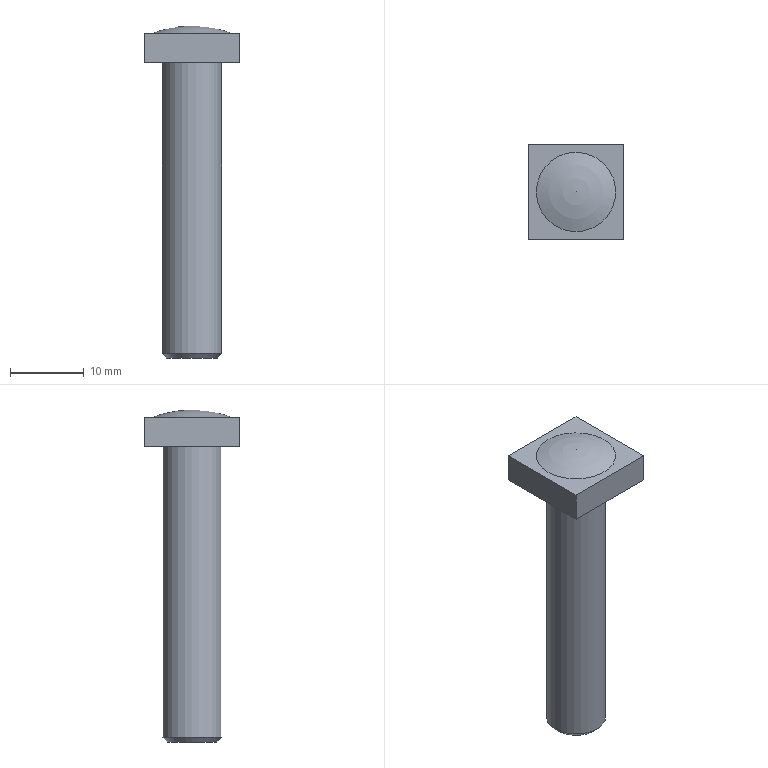Part | NX | features DATUM_CSYS 4, SKETCH 3, EXTRUDE 2, CHAMFER 1, SWP104 1 | 2 solids | 11 faces | box 13 x 13 x 45 mm | volume 2728 mm3 | plane 8 | sphere 1 | cylinder 1 | cone 1 | commonest cylinder face diameters 8 x1
STEP:
#1=CARTESIAN_POINT('',(-5.385,0.,4.));
#2=VERTEX_POINT('',#1);
#3=CARTESIAN_POINT('',(0.,0.,4.));
#4=DIRECTION('',(0.,0.,-1.));
#5=DIRECTION('',(-1.,0.,0.));
#6=AXIS2_PLACEMENT_3D('',#3,#4,#5);
#7=CIRCLE('',#6,5.385);
#8=EDGE_CURVE('',#2,#2,#7,.T.);
#9=ORIENTED_EDGE('',*,*,#8,.T.);
#10=EDGE_LOOP('',(#9));
#11=FACE_BOUND('',#10,.T.);
#12=CARTESIAN_POINT('',(0.,0.,4.));
#13=DIRECTION('',(0.,0.,-1.));
#14=DIRECTION('',(-1.,0.,0.));
#15=AXIS2_PLACEMENT_3D('',#12,#13,#14);
#16=PLANE('',#15);
#17=ADVANCED_FACE('',(#11),#16,.T.);
#18=ORIENTED_EDGE('',*,*,#8,.F.);
#19=EDGE_LOOP('',(#18));
#20=FACE_BOUND('',#19,.T.);
#21=CARTESIAN_POINT('',(0.,0.,-10.));
#22=DIRECTION('',(0.,0.,-1.));
#23=DIRECTION('',(0.,1.,0.));
#24=AXIS2_PLACEMENT_3D('',#21,#22,#23);
#25=SPHERICAL_SURFACE('',#24,15.);
#26=ADVANCED_FACE('',(#20),#25,.T.);
#27=CLOSED_SHELL('',(#17,#26));
#28=MANIFOLD_SOLID_BREP('',#27);
#29=CARTESIAN_POINT('',(-6.5,6.5,0.));
#30=VERTEX_POINT('',#29);
#31=CARTESIAN_POINT('',(-6.5,-6.5,0.));
#32=VERTEX_POINT('',#31);
#33=CARTESIAN_POINT('',(-6.5,6.5,0.));
#34=DIRECTION('',(0.,-1.,0.));
#35=VECTOR('',#34,1000.);
#36=LINE('',#33,#35);
#37=EDGE_CURVE('',#30,#32,#36,.T.);
#38=ORIENTED_EDGE('',*,*,#37,.T.);
#39=CARTESIAN_POINT('',(-6.5,-6.5,4.));
#40=VERTEX_POINT('',#39);
#41=CARTESIAN_POINT('',(-6.5,-6.5,4.));
#42=DIRECTION('',(0.,0.,-1.));
#43=VECTOR('',#42,1000.);
#44=LINE('',#41,#43);
#45=EDGE_CURVE('',#40,#32,#44,.T.);
#46=ORIENTED_EDGE('',*,*,#45,.F.);
#47=CARTESIAN_POINT('',(-6.5,6.5,4.));
#48=VERTEX_POINT('',#47);
#49=CARTESIAN_POINT('',(-6.5,6.5,4.));
#50=DIRECTION('',(0.,-1.,0.));
#51=VECTOR('',#50,1000.);
#52=LINE('',#49,#51);
#53=EDGE_CURVE('',#48,#40,#52,.T.);
#54=ORIENTED_EDGE('',*,*,#53,.F.);
#55=CARTESIAN_POINT('',(-6.5,6.5,4.));
#56=DIRECTION('',(0.,0.,-1.));
#57=VECTOR('',#56,1000.);
#58=LINE('',#55,#57);
#59=EDGE_CURVE('',#48,#30,#58,.T.);
#60=ORIENTED_EDGE('',*,*,#59,.T.);
#61=EDGE_LOOP('',(#38,#46,#54,#60));
#62=FACE_BOUND('',#61,.T.);
#63=CARTESIAN_POINT('',(-6.5,6.5,4.));
#64=DIRECTION('',(1.,0.,0.));
#65=DIRECTION('',(0.,0.,-1.));
#66=AXIS2_PLACEMENT_3D('',#63,#64,#65);
#67=PLANE('',#66);
#68=ADVANCED_FACE('',(#62),#67,.F.);
#69=CARTESIAN_POINT('',(6.5,-6.5,0.));
#70=VERTEX_POINT('',#69);
#71=CARTESIAN_POINT('',(-6.5,-6.5,0.));
#72=DIRECTION('',(1.,0.,0.));
#73=VECTOR('',#72,1000.);
#74=LINE('',#71,#73);
#75=EDGE_CURVE('',#32,#70,#74,.T.);
#76=ORIENTED_EDGE('',*,*,#75,.T.);
#77=CARTESIAN_POINT('',(6.5,-6.5,4.));
#78=VERTEX_POINT('',#77);
#79=CARTESIAN_POINT('',(6.5,-6.5,4.));
#80=DIRECTION('',(0.,0.,-1.));
#81=VECTOR('',#80,1000.);
#82=LINE('',#79,#81);
#83=EDGE_CURVE('',#78,#70,#82,.T.);
#84=ORIENTED_EDGE('',*,*,#83,.F.);
#85=CARTESIAN_POINT('',(-6.5,-6.5,4.));
#86=DIRECTION('',(1.,0.,0.));
#87=VECTOR('',#86,1000.);
#88=LINE('',#85,#87);
#89=EDGE_CURVE('',#40,#78,#88,.T.);
#90=ORIENTED_EDGE('',*,*,#89,.F.);
#91=ORIENTED_EDGE('',*,*,#45,.T.);
#92=EDGE_LOOP('',(#76,#84,#90,#91));
#93=FACE_BOUND('',#92,.T.);
#94=CARTESIAN_POINT('',(-6.5,-6.5,4.));
#95=DIRECTION('',(0.,1.,0.));
#96=DIRECTION('',(0.,0.,1.));
#97=AXIS2_PLACEMENT_3D('',#94,#95,#96);
#98=PLANE('',#97);
#99=ADVANCED_FACE('',(#93),#98,.F.);
#100=CARTESIAN_POINT('',(6.5,6.5,0.));
#101=VERTEX_POINT('',#100);
#102=CARTESIAN_POINT('',(6.5,-6.5,0.));
#103=DIRECTION('',(0.,1.,0.));
#104=VECTOR('',#103,1000.);
#105=LINE('',#102,#104);
#106=EDGE_CURVE('',#70,#101,#105,.T.);
#107=ORIENTED_EDGE('',*,*,#106,.T.);
#108=CARTESIAN_POINT('',(6.5,6.5,4.));
#109=VERTEX_POINT('',#108);
#110=CARTESIAN_POINT('',(6.5,6.5,4.));
#111=DIRECTION('',(0.,0.,-1.));
#112=VECTOR('',#111,1000.);
#113=LINE('',#110,#112);
#114=EDGE_CURVE('',#109,#101,#113,.T.);
#115=ORIENTED_EDGE('',*,*,#114,.F.);
#116=CARTESIAN_POINT('',(6.5,-6.5,4.));
#117=DIRECTION('',(0.,1.,0.));
#118=VECTOR('',#117,1000.);
#119=LINE('',#116,#118);
#120=EDGE_CURVE('',#78,#109,#119,.T.);
#121=ORIENTED_EDGE('',*,*,#120,.F.);
#122=ORIENTED_EDGE('',*,*,#83,.T.);
#123=EDGE_LOOP('',(#107,#115,#121,#122));
#124=FACE_BOUND('',#123,.T.);
#125=CARTESIAN_POINT('',(6.5,-6.5,4.));
#126=DIRECTION('',(-1.,0.,0.));
#127=DIRECTION('',(0.,0.,1.));
#128=AXIS2_PLACEMENT_3D('',#125,#126,#127);
#129=PLANE('',#128);
#130=ADVANCED_FACE('',(#124),#129,.F.);
#131=CARTESIAN_POINT('',(6.5,6.5,0.));
#132=DIRECTION('',(-1.,0.,0.));
#133=VECTOR('',#132,1000.);
#134=LINE('',#131,#133);
#135=EDGE_CURVE('',#101,#30,#134,.T.);
#136=ORIENTED_EDGE('',*,*,#135,.T.);
#137=ORIENTED_EDGE('',*,*,#59,.F.);
#138=CARTESIAN_POINT('',(6.5,6.5,4.));
#139=DIRECTION('',(-1.,0.,0.));
#140=VECTOR('',#139,1000.);
#141=LINE('',#138,#140);
#142=EDGE_CURVE('',#109,#48,#141,.T.);
#143=ORIENTED_EDGE('',*,*,#142,.F.);
#144=ORIENTED_EDGE('',*,*,#114,.T.);
#145=EDGE_LOOP('',(#136,#137,#143,#144));
#146=FACE_BOUND('',#145,.T.);
#147=CARTESIAN_POINT('',(6.5,6.5,4.));
#148=DIRECTION('',(0.,-1.,0.));
#149=DIRECTION('',(0.,0.,-1.));
#150=AXIS2_PLACEMENT_3D('',#147,#148,#149);
#151=PLANE('',#150);
#152=ADVANCED_FACE('',(#146),#151,.F.);
#153=ORIENTED_EDGE('',*,*,#53,.T.);
#154=ORIENTED_EDGE('',*,*,#89,.T.);
#155=ORIENTED_EDGE('',*,*,#120,.T.);
#156=ORIENTED_EDGE('',*,*,#142,.T.);
#157=EDGE_LOOP('',(#153,#154,#155,#156));
#158=FACE_BOUND('',#157,.T.);
#159=CARTESIAN_POINT('',(0.,0.,4.));
#160=DIRECTION('',(0.,0.,1.));
#161=DIRECTION('',(1.,0.,0.));
#162=AXIS2_PLACEMENT_3D('',#159,#160,#161);
#163=PLANE('',#162);
#164=ADVANCED_FACE('',(#158),#163,.T.);
#165=CARTESIAN_POINT('',(4.,0.,0.));
#166=VERTEX_POINT('',#165);
#167=CARTESIAN_POINT('',(0.,0.,0.));
#168=DIRECTION('',(0.,0.,-1.));
#169=DIRECTION('',(1.,0.,0.));
#170=AXIS2_PLACEMENT_3D('',#167,#168,#169);
#171=CIRCLE('',#170,4.);
#172=EDGE_CURVE('',#166,#166,#171,.T.);
#173=ORIENTED_EDGE('',*,*,#172,.F.);
#174=EDGE_LOOP('',(#173));
#175=FACE_BOUND('',#174,.T.);
#176=ORIENTED_EDGE('',*,*,#37,.F.);
#177=ORIENTED_EDGE('',*,*,#135,.F.);
#178=ORIENTED_EDGE('',*,*,#106,.F.);
#179=ORIENTED_EDGE('',*,*,#75,.F.);
#180=EDGE_LOOP('',(#176,#177,#178,#179));
#181=FACE_BOUND('',#180,.T.);
#182=CARTESIAN_POINT('',(0.,0.,0.));
#183=DIRECTION('',(0.,0.,1.));
#184=DIRECTION('',(1.,0.,0.));
#185=AXIS2_PLACEMENT_3D('',#182,#183,#184);
#186=PLANE('',#185);
#187=ADVANCED_FACE('',(#175,#181),#186,.F.);
#188=CARTESIAN_POINT('',(-4.,0.,-39.35));
#189=VERTEX_POINT('',#188);
#190=CARTESIAN_POINT('',(0.,0.,-39.35));
#191=DIRECTION('',(0.,0.,-1.));
#192=DIRECTION('',(-1.,0.,0.));
#193=AXIS2_PLACEMENT_3D('',#190,#191,#192);
#194=CIRCLE('',#193,4.);
#195=EDGE_CURVE('',#189,#189,#194,.F.);
#196=ORIENTED_EDGE('',*,*,#195,.T.);
#197=EDGE_LOOP('',(#196));
#198=FACE_BOUND('',#197,.T.);
#199=ORIENTED_EDGE('',*,*,#172,.T.);
#200=EDGE_LOOP('',(#199));
#201=FACE_BOUND('',#200,.T.);
#202=CARTESIAN_POINT('',(0.,0.,-40.));
#203=DIRECTION('',(0.,0.,1.));
#204=DIRECTION('',(1.,0.,0.));
#205=AXIS2_PLACEMENT_3D('',#202,#203,#204);
#206=CYLINDRICAL_SURFACE('',#205,4.);
#207=ADVANCED_FACE('',(#198,#201),#206,.T.);
#208=CARTESIAN_POINT('',(-3.4,0.,-40.));
#209=VERTEX_POINT('',#208);
#210=CARTESIAN_POINT('',(0.,0.,-40.));
#211=DIRECTION('',(0.,0.,-1.));
#212=DIRECTION('',(-1.,0.,0.));
#213=AXIS2_PLACEMENT_3D('',#210,#211,#212);
#214=CIRCLE('',#213,3.4);
#215=EDGE_CURVE('',#209,#209,#214,.T.);
#216=ORIENTED_EDGE('',*,*,#215,.T.);
#217=EDGE_LOOP('',(#216));
#218=FACE_BOUND('',#217,.T.);
#219=CARTESIAN_POINT('',(0.,0.,-40.));
#220=DIRECTION('',(0.,0.,-1.));
#221=DIRECTION('',(-1.,0.,0.));
#222=AXIS2_PLACEMENT_3D('',#219,#220,#221);
#223=PLANE('',#222);
#224=ADVANCED_FACE('',(#218),#223,.T.);
#225=ORIENTED_EDGE('',*,*,#195,.F.);
#226=EDGE_LOOP('',(#225));
#227=FACE_BOUND('',#226,.T.);
#228=ORIENTED_EDGE('',*,*,#215,.F.);
#229=EDGE_LOOP('',(#228));
#230=FACE_BOUND('',#229,.T.);
#231=CARTESIAN_POINT('',(0.,0.,-40.));
#232=DIRECTION('',(0.,0.,1.));
#233=DIRECTION('',(1.,0.,0.));
#234=AXIS2_PLACEMENT_3D('',#231,#232,#233);
#235=CONICAL_SURFACE('',#234,3.4,0.7454);
#236=ADVANCED_FACE('',(#227,#230),#235,.T.);
#237=CLOSED_SHELL('',(#68,#99,#130,#152,#164,#187,#207,#224,#236));
#238=MANIFOLD_SOLID_BREP('',#237);
#239=(LENGTH_UNIT()NAMED_UNIT(*)SI_UNIT(.MILLI.,.METRE.));
#240=UNCERTAINTY_MEASURE_WITH_UNIT(LENGTH_MEASURE(0.00001),#239,'','');
#241=(NAMED_UNIT(*)PLANE_ANGLE_UNIT()SI_UNIT($,.RADIAN.));
#242=(NAMED_UNIT(*)SI_UNIT($,.STERADIAN.)SOLID_ANGLE_UNIT());
#243=(GEOMETRIC_REPRESENTATION_CONTEXT(3)GLOBAL_UNCERTAINTY_ASSIGNED_CONTEXT((#240))GLOBAL_UNIT_ASSIGNED_CONTEXT((#239,#241,#242))REPRESENTATION_CONTEXT('',''));
#244=ADVANCED_BREP_SHAPE_REPRESENTATION('',(#28,#238),#243);